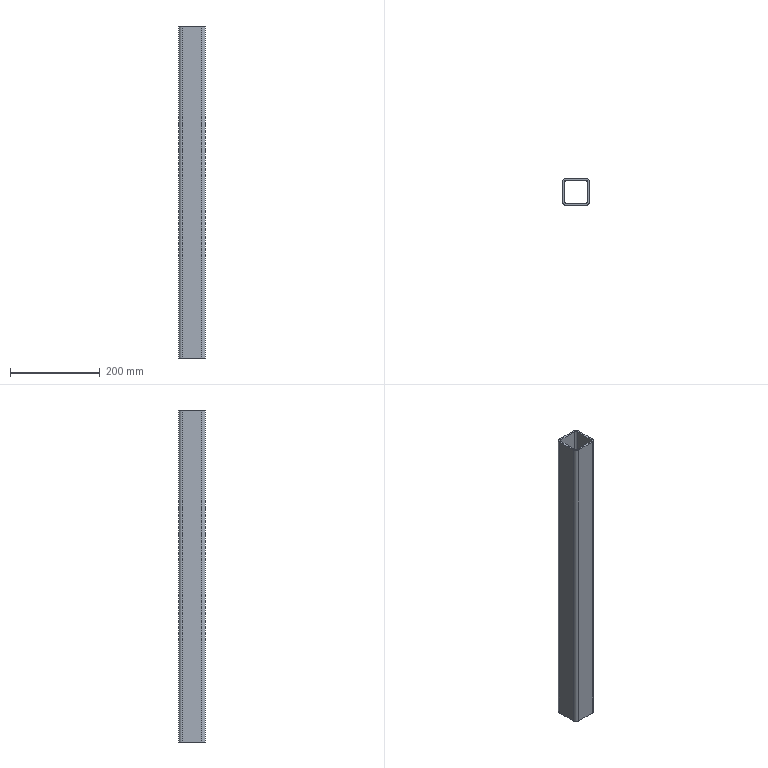Part | SolidWorks | features ICE 1, LibraryFeature 1 | 1 solid | 18 faces | box 60 x 60 x 740 mm | volume 632549 mm3 | plane 10 | cylinder 8 | commonest cylinder face diameters 8 x4 16 x4
STEP:
#1=CARTESIAN_POINT('',(22.,30.,0.));
#2=VERTEX_POINT('',#1);
#3=CARTESIAN_POINT('',(-22.,30.,0.));
#4=VERTEX_POINT('',#3);
#5=CARTESIAN_POINT('',(0.,30.,0.));
#6=DIRECTION('',(-1.,0.,0.));
#7=VECTOR('',#6,1000.);
#8=LINE('',#5,#7);
#9=EDGE_CURVE('',#2,#4,#8,.T.);
#10=ORIENTED_EDGE('',*,*,#9,.T.);
#11=CARTESIAN_POINT('',(-22.,30.,740.));
#12=VERTEX_POINT('',#11);
#13=CARTESIAN_POINT('',(-22.,30.,740.));
#14=DIRECTION('',(0.,0.,-1.));
#15=VECTOR('',#14,1000.);
#16=LINE('',#13,#15);
#17=EDGE_CURVE('',#12,#4,#16,.T.);
#18=ORIENTED_EDGE('',*,*,#17,.F.);
#19=CARTESIAN_POINT('',(22.,30.,740.));
#20=VERTEX_POINT('',#19);
#21=CARTESIAN_POINT('',(0.,30.,740.));
#22=DIRECTION('',(-1.,0.,0.));
#23=VECTOR('',#22,1000.);
#24=LINE('',#21,#23);
#25=EDGE_CURVE('',#20,#12,#24,.T.);
#26=ORIENTED_EDGE('',*,*,#25,.F.);
#27=CARTESIAN_POINT('',(22.,30.,740.));
#28=DIRECTION('',(0.,0.,-1.));
#29=VECTOR('',#28,1000.);
#30=LINE('',#27,#29);
#31=EDGE_CURVE('',#20,#2,#30,.T.);
#32=ORIENTED_EDGE('',*,*,#31,.T.);
#33=EDGE_LOOP('',(#10,#18,#26,#32));
#34=FACE_OUTER_BOUND('',#33,.T.);
#35=CARTESIAN_POINT('',(0.,30.,740.));
#36=DIRECTION('',(0.,-1.,0.));
#37=DIRECTION('',(0.,0.,-1.));
#38=AXIS2_PLACEMENT_3D('',#35,#36,#37);
#39=PLANE('',#38);
#40=ADVANCED_FACE('',(#34),#39,.F.);
#41=CARTESIAN_POINT('',(-30.,22.,0.));
#42=VERTEX_POINT('',#41);
#43=CARTESIAN_POINT('',(-22.,22.,0.));
#44=DIRECTION('',(0.,0.,1.));
#45=DIRECTION('',(1.,0.,0.));
#46=AXIS2_PLACEMENT_3D('',#43,#44,#45);
#47=CIRCLE('',#46,8.);
#48=EDGE_CURVE('',#4,#42,#47,.T.);
#49=ORIENTED_EDGE('',*,*,#48,.T.);
#50=CARTESIAN_POINT('',(-30.,22.,740.));
#51=VERTEX_POINT('',#50);
#52=CARTESIAN_POINT('',(-30.,22.,740.));
#53=DIRECTION('',(0.,0.,-1.));
#54=VECTOR('',#53,1000.);
#55=LINE('',#52,#54);
#56=EDGE_CURVE('',#51,#42,#55,.T.);
#57=ORIENTED_EDGE('',*,*,#56,.F.);
#58=CARTESIAN_POINT('',(-22.,22.,740.));
#59=DIRECTION('',(0.,0.,1.));
#60=DIRECTION('',(1.,0.,0.));
#61=AXIS2_PLACEMENT_3D('',#58,#59,#60);
#62=CIRCLE('',#61,8.);
#63=EDGE_CURVE('',#12,#51,#62,.T.);
#64=ORIENTED_EDGE('',*,*,#63,.F.);
#65=ORIENTED_EDGE('',*,*,#17,.T.);
#66=EDGE_LOOP('',(#49,#57,#64,#65));
#67=FACE_OUTER_BOUND('',#66,.T.);
#68=CARTESIAN_POINT('',(-22.,22.,740.));
#69=DIRECTION('',(0.,0.,-1.));
#70=DIRECTION('',(-1.,0.,0.));
#71=AXIS2_PLACEMENT_3D('',#68,#69,#70);
#72=CYLINDRICAL_SURFACE('',#71,8.);
#73=ADVANCED_FACE('',(#67),#72,.T.);
#74=CARTESIAN_POINT('',(-30.,-22.,0.));
#75=VERTEX_POINT('',#74);
#76=CARTESIAN_POINT('',(-30.,0.,0.));
#77=DIRECTION('',(0.,1.,0.));
#78=VECTOR('',#77,1000.);
#79=LINE('',#76,#78);
#80=EDGE_CURVE('',#75,#42,#79,.T.);
#81=ORIENTED_EDGE('',*,*,#80,.F.);
#82=CARTESIAN_POINT('',(-30.,-22.,740.));
#83=VERTEX_POINT('',#82);
#84=CARTESIAN_POINT('',(-30.,-22.,740.));
#85=DIRECTION('',(0.,0.,-1.));
#86=VECTOR('',#85,1000.);
#87=LINE('',#84,#86);
#88=EDGE_CURVE('',#83,#75,#87,.T.);
#89=ORIENTED_EDGE('',*,*,#88,.F.);
#90=CARTESIAN_POINT('',(-30.,0.,740.));
#91=DIRECTION('',(0.,1.,0.));
#92=VECTOR('',#91,1000.);
#93=LINE('',#90,#92);
#94=EDGE_CURVE('',#83,#51,#93,.T.);
#95=ORIENTED_EDGE('',*,*,#94,.T.);
#96=ORIENTED_EDGE('',*,*,#56,.T.);
#97=EDGE_LOOP('',(#81,#89,#95,#96));
#98=FACE_OUTER_BOUND('',#97,.T.);
#99=CARTESIAN_POINT('',(-30.,0.,740.));
#100=DIRECTION('',(-1.,0.,0.));
#101=DIRECTION('',(0.,0.,1.));
#102=AXIS2_PLACEMENT_3D('',#99,#100,#101);
#103=PLANE('',#102);
#104=ADVANCED_FACE('',(#98),#103,.T.);
#105=CARTESIAN_POINT('',(-22.,-30.,0.));
#106=VERTEX_POINT('',#105);
#107=CARTESIAN_POINT('',(-22.,-22.,0.));
#108=DIRECTION('',(0.,0.,1.));
#109=DIRECTION('',(1.,0.,0.));
#110=AXIS2_PLACEMENT_3D('',#107,#108,#109);
#111=CIRCLE('',#110,8.);
#112=EDGE_CURVE('',#75,#106,#111,.T.);
#113=ORIENTED_EDGE('',*,*,#112,.T.);
#114=CARTESIAN_POINT('',(-22.,-30.,740.));
#115=VERTEX_POINT('',#114);
#116=CARTESIAN_POINT('',(-22.,-30.,740.));
#117=DIRECTION('',(0.,0.,-1.));
#118=VECTOR('',#117,1000.);
#119=LINE('',#116,#118);
#120=EDGE_CURVE('',#115,#106,#119,.T.);
#121=ORIENTED_EDGE('',*,*,#120,.F.);
#122=CARTESIAN_POINT('',(-22.,-22.,740.));
#123=DIRECTION('',(0.,0.,1.));
#124=DIRECTION('',(1.,0.,0.));
#125=AXIS2_PLACEMENT_3D('',#122,#123,#124);
#126=CIRCLE('',#125,8.);
#127=EDGE_CURVE('',#83,#115,#126,.T.);
#128=ORIENTED_EDGE('',*,*,#127,.F.);
#129=ORIENTED_EDGE('',*,*,#88,.T.);
#130=EDGE_LOOP('',(#113,#121,#128,#129));
#131=FACE_OUTER_BOUND('',#130,.T.);
#132=CARTESIAN_POINT('',(-22.,-22.,740.));
#133=DIRECTION('',(0.,0.,-1.));
#134=DIRECTION('',(-1.,0.,0.));
#135=AXIS2_PLACEMENT_3D('',#132,#133,#134);
#136=CYLINDRICAL_SURFACE('',#135,8.);
#137=ADVANCED_FACE('',(#131),#136,.T.);
#138=CARTESIAN_POINT('',(22.,-30.,0.));
#139=VERTEX_POINT('',#138);
#140=CARTESIAN_POINT('',(0.,-30.,0.));
#141=DIRECTION('',(1.,0.,0.));
#142=VECTOR('',#141,1000.);
#143=LINE('',#140,#142);
#144=EDGE_CURVE('',#106,#139,#143,.T.);
#145=ORIENTED_EDGE('',*,*,#144,.T.);
#146=CARTESIAN_POINT('',(22.,-30.,740.));
#147=VERTEX_POINT('',#146);
#148=CARTESIAN_POINT('',(22.,-30.,740.));
#149=DIRECTION('',(0.,0.,-1.));
#150=VECTOR('',#149,1000.);
#151=LINE('',#148,#150);
#152=EDGE_CURVE('',#147,#139,#151,.T.);
#153=ORIENTED_EDGE('',*,*,#152,.F.);
#154=CARTESIAN_POINT('',(0.,-30.,740.));
#155=DIRECTION('',(1.,0.,0.));
#156=VECTOR('',#155,1000.);
#157=LINE('',#154,#156);
#158=EDGE_CURVE('',#115,#147,#157,.T.);
#159=ORIENTED_EDGE('',*,*,#158,.F.);
#160=ORIENTED_EDGE('',*,*,#120,.T.);
#161=EDGE_LOOP('',(#145,#153,#159,#160));
#162=FACE_OUTER_BOUND('',#161,.T.);
#163=CARTESIAN_POINT('',(0.,-30.,740.));
#164=DIRECTION('',(0.,1.,0.));
#165=DIRECTION('',(0.,0.,1.));
#166=AXIS2_PLACEMENT_3D('',#163,#164,#165);
#167=PLANE('',#166);
#168=ADVANCED_FACE('',(#162),#167,.F.);
#169=CARTESIAN_POINT('',(30.,-22.,0.));
#170=VERTEX_POINT('',#169);
#171=CARTESIAN_POINT('',(22.,-22.,0.));
#172=DIRECTION('',(0.,0.,1.));
#173=DIRECTION('',(1.,0.,0.));
#174=AXIS2_PLACEMENT_3D('',#171,#172,#173);
#175=CIRCLE('',#174,8.);
#176=EDGE_CURVE('',#139,#170,#175,.T.);
#177=ORIENTED_EDGE('',*,*,#176,.T.);
#178=CARTESIAN_POINT('',(30.,-22.,740.));
#179=VERTEX_POINT('',#178);
#180=CARTESIAN_POINT('',(30.,-22.,740.));
#181=DIRECTION('',(0.,0.,-1.));
#182=VECTOR('',#181,1000.);
#183=LINE('',#180,#182);
#184=EDGE_CURVE('',#179,#170,#183,.T.);
#185=ORIENTED_EDGE('',*,*,#184,.F.);
#186=CARTESIAN_POINT('',(22.,-22.,740.));
#187=DIRECTION('',(0.,0.,1.));
#188=DIRECTION('',(1.,0.,0.));
#189=AXIS2_PLACEMENT_3D('',#186,#187,#188);
#190=CIRCLE('',#189,8.);
#191=EDGE_CURVE('',#147,#179,#190,.T.);
#192=ORIENTED_EDGE('',*,*,#191,.F.);
#193=ORIENTED_EDGE('',*,*,#152,.T.);
#194=EDGE_LOOP('',(#177,#185,#192,#193));
#195=FACE_OUTER_BOUND('',#194,.T.);
#196=CARTESIAN_POINT('',(22.,-22.,740.));
#197=DIRECTION('',(0.,0.,-1.));
#198=DIRECTION('',(-1.,0.,0.));
#199=AXIS2_PLACEMENT_3D('',#196,#197,#198);
#200=CYLINDRICAL_SURFACE('',#199,8.);
#201=ADVANCED_FACE('',(#195),#200,.T.);
#202=CARTESIAN_POINT('',(30.,22.,0.));
#203=VERTEX_POINT('',#202);
#204=CARTESIAN_POINT('',(30.,0.,0.));
#205=DIRECTION('',(0.,-1.,0.));
#206=VECTOR('',#205,1000.);
#207=LINE('',#204,#206);
#208=EDGE_CURVE('',#203,#170,#207,.T.);
#209=ORIENTED_EDGE('',*,*,#208,.F.);
#210=CARTESIAN_POINT('',(30.,22.,740.));
#211=VERTEX_POINT('',#210);
#212=CARTESIAN_POINT('',(30.,22.,740.));
#213=DIRECTION('',(0.,0.,-1.));
#214=VECTOR('',#213,1000.);
#215=LINE('',#212,#214);
#216=EDGE_CURVE('',#211,#203,#215,.T.);
#217=ORIENTED_EDGE('',*,*,#216,.F.);
#218=CARTESIAN_POINT('',(30.,0.,740.));
#219=DIRECTION('',(0.,-1.,0.));
#220=VECTOR('',#219,1000.);
#221=LINE('',#218,#220);
#222=EDGE_CURVE('',#211,#179,#221,.T.);
#223=ORIENTED_EDGE('',*,*,#222,.T.);
#224=ORIENTED_EDGE('',*,*,#184,.T.);
#225=EDGE_LOOP('',(#209,#217,#223,#224));
#226=FACE_OUTER_BOUND('',#225,.T.);
#227=CARTESIAN_POINT('',(30.,0.,740.));
#228=DIRECTION('',(1.,0.,0.));
#229=DIRECTION('',(0.,0.,-1.));
#230=AXIS2_PLACEMENT_3D('',#227,#228,#229);
#231=PLANE('',#230);
#232=ADVANCED_FACE('',(#226),#231,.T.);
#233=CARTESIAN_POINT('',(-26.,-22.,0.));
#234=VERTEX_POINT('',#233);
#235=CARTESIAN_POINT('',(-22.,-26.,0.));
#236=VERTEX_POINT('',#235);
#237=CARTESIAN_POINT('',(-22.,-22.,0.));
#238=DIRECTION('',(0.,0.,1.));
#239=DIRECTION('',(1.,0.,0.));
#240=AXIS2_PLACEMENT_3D('',#237,#238,#239);
#241=CIRCLE('',#240,4.);
#242=EDGE_CURVE('',#234,#236,#241,.T.);
#243=ORIENTED_EDGE('',*,*,#242,.F.);
#244=CARTESIAN_POINT('',(-26.,-22.,740.));
#245=VERTEX_POINT('',#244);
#246=CARTESIAN_POINT('',(-26.,-22.,740.));
#247=DIRECTION('',(0.,0.,-1.));
#248=VECTOR('',#247,1000.);
#249=LINE('',#246,#248);
#250=EDGE_CURVE('',#245,#234,#249,.T.);
#251=ORIENTED_EDGE('',*,*,#250,.F.);
#252=CARTESIAN_POINT('',(-22.,-26.,740.));
#253=VERTEX_POINT('',#252);
#254=CARTESIAN_POINT('',(-22.,-22.,740.));
#255=DIRECTION('',(0.,0.,1.));
#256=DIRECTION('',(1.,0.,0.));
#257=AXIS2_PLACEMENT_3D('',#254,#255,#256);
#258=CIRCLE('',#257,4.);
#259=EDGE_CURVE('',#245,#253,#258,.T.);
#260=ORIENTED_EDGE('',*,*,#259,.T.);
#261=CARTESIAN_POINT('',(-22.,-26.,740.));
#262=DIRECTION('',(0.,0.,-1.));
#263=VECTOR('',#262,1000.);
#264=LINE('',#261,#263);
#265=EDGE_CURVE('',#253,#236,#264,.T.);
#266=ORIENTED_EDGE('',*,*,#265,.T.);
#267=EDGE_LOOP('',(#243,#251,#260,#266));
#268=FACE_OUTER_BOUND('',#267,.T.);
#269=CARTESIAN_POINT('',(-22.,-22.,740.));
#270=DIRECTION('',(0.,0.,-1.));
#271=DIRECTION('',(-1.,0.,0.));
#272=AXIS2_PLACEMENT_3D('',#269,#270,#271);
#273=CYLINDRICAL_SURFACE('',#272,4.);
#274=ADVANCED_FACE('',(#268),#273,.F.);
#275=CARTESIAN_POINT('',(-26.,22.,0.));
#276=VERTEX_POINT('',#275);
#277=CARTESIAN_POINT('',(-26.,0.,0.));
#278=DIRECTION('',(0.,1.,0.));
#279=VECTOR('',#278,1000.);
#280=LINE('',#277,#279);
#281=EDGE_CURVE('',#234,#276,#280,.T.);
#282=ORIENTED_EDGE('',*,*,#281,.T.);
#283=CARTESIAN_POINT('',(-26.,22.,740.));
#284=VERTEX_POINT('',#283);
#285=CARTESIAN_POINT('',(-26.,22.,740.));
#286=DIRECTION('',(0.,0.,-1.));
#287=VECTOR('',#286,1000.);
#288=LINE('',#285,#287);
#289=EDGE_CURVE('',#284,#276,#288,.T.);
#290=ORIENTED_EDGE('',*,*,#289,.F.);
#291=CARTESIAN_POINT('',(-26.,0.,740.));
#292=DIRECTION('',(0.,1.,0.));
#293=VECTOR('',#292,1000.);
#294=LINE('',#291,#293);
#295=EDGE_CURVE('',#245,#284,#294,.T.);
#296=ORIENTED_EDGE('',*,*,#295,.F.);
#297=ORIENTED_EDGE('',*,*,#250,.T.);
#298=EDGE_LOOP('',(#282,#290,#296,#297));
#299=FACE_OUTER_BOUND('',#298,.T.);
#300=CARTESIAN_POINT('',(-26.,0.,740.));
#301=DIRECTION('',(-1.,0.,0.));
#302=DIRECTION('',(0.,0.,1.));
#303=AXIS2_PLACEMENT_3D('',#300,#301,#302);
#304=PLANE('',#303);
#305=ADVANCED_FACE('',(#299),#304,.F.);
#306=CARTESIAN_POINT('',(-22.,26.,0.));
#307=VERTEX_POINT('',#306);
#308=CARTESIAN_POINT('',(-22.,22.,0.));
#309=DIRECTION('',(0.,0.,1.));
#310=DIRECTION('',(1.,0.,0.));
#311=AXIS2_PLACEMENT_3D('',#308,#309,#310);
#312=CIRCLE('',#311,4.);
#313=EDGE_CURVE('',#307,#276,#312,.T.);
#314=ORIENTED_EDGE('',*,*,#313,.F.);
#315=CARTESIAN_POINT('',(-22.,26.,740.));
#316=VERTEX_POINT('',#315);
#317=CARTESIAN_POINT('',(-22.,26.,740.));
#318=DIRECTION('',(0.,0.,-1.));
#319=VECTOR('',#318,1000.);
#320=LINE('',#317,#319);
#321=EDGE_CURVE('',#316,#307,#320,.T.);
#322=ORIENTED_EDGE('',*,*,#321,.F.);
#323=CARTESIAN_POINT('',(-22.,22.,740.));
#324=DIRECTION('',(0.,0.,1.));
#325=DIRECTION('',(1.,0.,0.));
#326=AXIS2_PLACEMENT_3D('',#323,#324,#325);
#327=CIRCLE('',#326,4.);
#328=EDGE_CURVE('',#316,#284,#327,.T.);
#329=ORIENTED_EDGE('',*,*,#328,.T.);
#330=ORIENTED_EDGE('',*,*,#289,.T.);
#331=EDGE_LOOP('',(#314,#322,#329,#330));
#332=FACE_OUTER_BOUND('',#331,.T.);
#333=CARTESIAN_POINT('',(-22.,22.,740.));
#334=DIRECTION('',(0.,0.,-1.));
#335=DIRECTION('',(-1.,0.,0.));
#336=AXIS2_PLACEMENT_3D('',#333,#334,#335);
#337=CYLINDRICAL_SURFACE('',#336,4.);
#338=ADVANCED_FACE('',(#332),#337,.F.);
#339=CARTESIAN_POINT('',(22.,26.,0.));
#340=VERTEX_POINT('',#339);
#341=CARTESIAN_POINT('',(0.,26.,0.));
#342=DIRECTION('',(-1.,0.,0.));
#343=VECTOR('',#342,1000.);
#344=LINE('',#341,#343);
#345=EDGE_CURVE('',#340,#307,#344,.T.);
#346=ORIENTED_EDGE('',*,*,#345,.F.);
#347=CARTESIAN_POINT('',(22.,26.,740.));
#348=VERTEX_POINT('',#347);
#349=CARTESIAN_POINT('',(22.,26.,740.));
#350=DIRECTION('',(0.,0.,-1.));
#351=VECTOR('',#350,1000.);
#352=LINE('',#349,#351);
#353=EDGE_CURVE('',#348,#340,#352,.T.);
#354=ORIENTED_EDGE('',*,*,#353,.F.);
#355=CARTESIAN_POINT('',(0.,26.,740.));
#356=DIRECTION('',(-1.,0.,0.));
#357=VECTOR('',#356,1000.);
#358=LINE('',#355,#357);
#359=EDGE_CURVE('',#348,#316,#358,.T.);
#360=ORIENTED_EDGE('',*,*,#359,.T.);
#361=ORIENTED_EDGE('',*,*,#321,.T.);
#362=EDGE_LOOP('',(#346,#354,#360,#361));
#363=FACE_OUTER_BOUND('',#362,.T.);
#364=CARTESIAN_POINT('',(0.,26.,740.));
#365=DIRECTION('',(0.,-1.,0.));
#366=DIRECTION('',(0.,0.,-1.));
#367=AXIS2_PLACEMENT_3D('',#364,#365,#366);
#368=PLANE('',#367);
#369=ADVANCED_FACE('',(#363),#368,.T.);
#370=CARTESIAN_POINT('',(26.,22.,0.));
#371=VERTEX_POINT('',#370);
#372=CARTESIAN_POINT('',(22.,22.,0.));
#373=DIRECTION('',(0.,0.,1.));
#374=DIRECTION('',(1.,0.,0.));
#375=AXIS2_PLACEMENT_3D('',#372,#373,#374);
#376=CIRCLE('',#375,4.);
#377=EDGE_CURVE('',#371,#340,#376,.T.);
#378=ORIENTED_EDGE('',*,*,#377,.F.);
#379=CARTESIAN_POINT('',(26.,22.,740.));
#380=VERTEX_POINT('',#379);
#381=CARTESIAN_POINT('',(26.,22.,740.));
#382=DIRECTION('',(0.,0.,-1.));
#383=VECTOR('',#382,1000.);
#384=LINE('',#381,#383);
#385=EDGE_CURVE('',#380,#371,#384,.T.);
#386=ORIENTED_EDGE('',*,*,#385,.F.);
#387=CARTESIAN_POINT('',(22.,22.,740.));
#388=DIRECTION('',(0.,0.,1.));
#389=DIRECTION('',(1.,0.,0.));
#390=AXIS2_PLACEMENT_3D('',#387,#388,#389);
#391=CIRCLE('',#390,4.);
#392=EDGE_CURVE('',#380,#348,#391,.T.);
#393=ORIENTED_EDGE('',*,*,#392,.T.);
#394=ORIENTED_EDGE('',*,*,#353,.T.);
#395=EDGE_LOOP('',(#378,#386,#393,#394));
#396=FACE_OUTER_BOUND('',#395,.T.);
#397=CARTESIAN_POINT('',(22.,22.,740.));
#398=DIRECTION('',(0.,0.,-1.));
#399=DIRECTION('',(-1.,0.,0.));
#400=AXIS2_PLACEMENT_3D('',#397,#398,#399);
#401=CYLINDRICAL_SURFACE('',#400,4.);
#402=ADVANCED_FACE('',(#396),#401,.F.);
#403=CARTESIAN_POINT('',(26.,-22.,0.));
#404=VERTEX_POINT('',#403);
#405=CARTESIAN_POINT('',(26.,0.,0.));
#406=DIRECTION('',(0.,-1.,0.));
#407=VECTOR('',#406,1000.);
#408=LINE('',#405,#407);
#409=EDGE_CURVE('',#371,#404,#408,.T.);
#410=ORIENTED_EDGE('',*,*,#409,.T.);
#411=CARTESIAN_POINT('',(26.,-22.,740.));
#412=VERTEX_POINT('',#411);
#413=CARTESIAN_POINT('',(26.,-22.,740.));
#414=DIRECTION('',(0.,0.,-1.));
#415=VECTOR('',#414,1000.);
#416=LINE('',#413,#415);
#417=EDGE_CURVE('',#412,#404,#416,.T.);
#418=ORIENTED_EDGE('',*,*,#417,.F.);
#419=CARTESIAN_POINT('',(26.,0.,740.));
#420=DIRECTION('',(0.,-1.,0.));
#421=VECTOR('',#420,1000.);
#422=LINE('',#419,#421);
#423=EDGE_CURVE('',#380,#412,#422,.T.);
#424=ORIENTED_EDGE('',*,*,#423,.F.);
#425=ORIENTED_EDGE('',*,*,#385,.T.);
#426=EDGE_LOOP('',(#410,#418,#424,#425));
#427=FACE_OUTER_BOUND('',#426,.T.);
#428=CARTESIAN_POINT('',(26.,0.,740.));
#429=DIRECTION('',(1.,0.,0.));
#430=DIRECTION('',(0.,0.,-1.));
#431=AXIS2_PLACEMENT_3D('',#428,#429,#430);
#432=PLANE('',#431);
#433=ADVANCED_FACE('',(#427),#432,.F.);
#434=CARTESIAN_POINT('',(22.,-26.,0.));
#435=VERTEX_POINT('',#434);
#436=CARTESIAN_POINT('',(22.,-22.,0.));
#437=DIRECTION('',(0.,0.,1.));
#438=DIRECTION('',(1.,0.,0.));
#439=AXIS2_PLACEMENT_3D('',#436,#437,#438);
#440=CIRCLE('',#439,4.);
#441=EDGE_CURVE('',#435,#404,#440,.T.);
#442=ORIENTED_EDGE('',*,*,#441,.F.);
#443=CARTESIAN_POINT('',(22.,-26.,740.));
#444=VERTEX_POINT('',#443);
#445=CARTESIAN_POINT('',(22.,-26.,740.));
#446=DIRECTION('',(0.,0.,-1.));
#447=VECTOR('',#446,1000.);
#448=LINE('',#445,#447);
#449=EDGE_CURVE('',#444,#435,#448,.T.);
#450=ORIENTED_EDGE('',*,*,#449,.F.);
#451=CARTESIAN_POINT('',(22.,-22.,740.));
#452=DIRECTION('',(0.,0.,1.));
#453=DIRECTION('',(1.,0.,0.));
#454=AXIS2_PLACEMENT_3D('',#451,#452,#453);
#455=CIRCLE('',#454,4.);
#456=EDGE_CURVE('',#444,#412,#455,.T.);
#457=ORIENTED_EDGE('',*,*,#456,.T.);
#458=ORIENTED_EDGE('',*,*,#417,.T.);
#459=EDGE_LOOP('',(#442,#450,#457,#458));
#460=FACE_OUTER_BOUND('',#459,.T.);
#461=CARTESIAN_POINT('',(22.,-22.,740.));
#462=DIRECTION('',(0.,0.,-1.));
#463=DIRECTION('',(-1.,0.,0.));
#464=AXIS2_PLACEMENT_3D('',#461,#462,#463);
#465=CYLINDRICAL_SURFACE('',#464,4.);
#466=ADVANCED_FACE('',(#460),#465,.F.);
#467=CARTESIAN_POINT('',(0.,-26.,0.));
#468=DIRECTION('',(1.,0.,0.));
#469=VECTOR('',#468,1000.);
#470=LINE('',#467,#469);
#471=EDGE_CURVE('',#236,#435,#470,.T.);
#472=ORIENTED_EDGE('',*,*,#471,.F.);
#473=ORIENTED_EDGE('',*,*,#265,.F.);
#474=CARTESIAN_POINT('',(0.,-26.,740.));
#475=DIRECTION('',(1.,0.,0.));
#476=VECTOR('',#475,1000.);
#477=LINE('',#474,#476);
#478=EDGE_CURVE('',#253,#444,#477,.T.);
#479=ORIENTED_EDGE('',*,*,#478,.T.);
#480=ORIENTED_EDGE('',*,*,#449,.T.);
#481=EDGE_LOOP('',(#472,#473,#479,#480));
#482=FACE_OUTER_BOUND('',#481,.T.);
#483=CARTESIAN_POINT('',(0.,-26.,740.));
#484=DIRECTION('',(0.,1.,0.));
#485=DIRECTION('',(0.,0.,1.));
#486=AXIS2_PLACEMENT_3D('',#483,#484,#485);
#487=PLANE('',#486);
#488=ADVANCED_FACE('',(#482),#487,.T.);
#489=CARTESIAN_POINT('',(22.,22.,0.));
#490=DIRECTION('',(0.,0.,1.));
#491=DIRECTION('',(1.,0.,0.));
#492=AXIS2_PLACEMENT_3D('',#489,#490,#491);
#493=CIRCLE('',#492,8.);
#494=EDGE_CURVE('',#203,#2,#493,.T.);
#495=ORIENTED_EDGE('',*,*,#494,.T.);
#496=ORIENTED_EDGE('',*,*,#31,.F.);
#497=CARTESIAN_POINT('',(22.,22.,740.));
#498=DIRECTION('',(0.,0.,1.));
#499=DIRECTION('',(1.,0.,0.));
#500=AXIS2_PLACEMENT_3D('',#497,#498,#499);
#501=CIRCLE('',#500,8.);
#502=EDGE_CURVE('',#211,#20,#501,.T.);
#503=ORIENTED_EDGE('',*,*,#502,.F.);
#504=ORIENTED_EDGE('',*,*,#216,.T.);
#505=EDGE_LOOP('',(#495,#496,#503,#504));
#506=FACE_OUTER_BOUND('',#505,.T.);
#507=CARTESIAN_POINT('',(22.,22.,740.));
#508=DIRECTION('',(0.,0.,-1.));
#509=DIRECTION('',(-1.,0.,0.));
#510=AXIS2_PLACEMENT_3D('',#507,#508,#509);
#511=CYLINDRICAL_SURFACE('',#510,8.);
#512=ADVANCED_FACE('',(#506),#511,.T.);
#513=ORIENTED_EDGE('',*,*,#259,.F.);
#514=ORIENTED_EDGE('',*,*,#295,.T.);
#515=ORIENTED_EDGE('',*,*,#328,.F.);
#516=ORIENTED_EDGE('',*,*,#359,.F.);
#517=ORIENTED_EDGE('',*,*,#392,.F.);
#518=ORIENTED_EDGE('',*,*,#423,.T.);
#519=ORIENTED_EDGE('',*,*,#456,.F.);
#520=ORIENTED_EDGE('',*,*,#478,.F.);
#521=EDGE_LOOP('',(#513,#514,#515,#516,#517,#518,#519,#520));
#522=FACE_BOUND('',#521,.T.);
#523=ORIENTED_EDGE('',*,*,#25,.T.);
#524=ORIENTED_EDGE('',*,*,#63,.T.);
#525=ORIENTED_EDGE('',*,*,#94,.F.);
#526=ORIENTED_EDGE('',*,*,#127,.T.);
#527=ORIENTED_EDGE('',*,*,#158,.T.);
#528=ORIENTED_EDGE('',*,*,#191,.T.);
#529=ORIENTED_EDGE('',*,*,#222,.F.);
#530=ORIENTED_EDGE('',*,*,#502,.T.);
#531=EDGE_LOOP('',(#523,#524,#525,#526,#527,#528,#529,#530));
#532=FACE_OUTER_BOUND('',#531,.T.);
#533=CARTESIAN_POINT('',(0.,0.,740.));
#534=DIRECTION('',(0.,0.,1.));
#535=DIRECTION('',(1.,0.,0.));
#536=AXIS2_PLACEMENT_3D('',#533,#534,#535);
#537=PLANE('',#536);
#538=ADVANCED_FACE('',(#522,#532),#537,.T.);
#539=ORIENTED_EDGE('',*,*,#242,.T.);
#540=ORIENTED_EDGE('',*,*,#471,.T.);
#541=ORIENTED_EDGE('',*,*,#441,.T.);
#542=ORIENTED_EDGE('',*,*,#409,.F.);
#543=ORIENTED_EDGE('',*,*,#377,.T.);
#544=ORIENTED_EDGE('',*,*,#345,.T.);
#545=ORIENTED_EDGE('',*,*,#313,.T.);
#546=ORIENTED_EDGE('',*,*,#281,.F.);
#547=EDGE_LOOP('',(#539,#540,#541,#542,#543,#544,#545,#546));
#548=FACE_BOUND('',#547,.T.);
#549=ORIENTED_EDGE('',*,*,#9,.F.);
#550=ORIENTED_EDGE('',*,*,#494,.F.);
#551=ORIENTED_EDGE('',*,*,#208,.T.);
#552=ORIENTED_EDGE('',*,*,#176,.F.);
#553=ORIENTED_EDGE('',*,*,#144,.F.);
#554=ORIENTED_EDGE('',*,*,#112,.F.);
#555=ORIENTED_EDGE('',*,*,#80,.T.);
#556=ORIENTED_EDGE('',*,*,#48,.F.);
#557=EDGE_LOOP('',(#549,#550,#551,#552,#553,#554,#555,#556));
#558=FACE_OUTER_BOUND('',#557,.T.);
#559=CARTESIAN_POINT('',(0.,0.,0.));
#560=DIRECTION('',(0.,0.,1.));
#561=DIRECTION('',(1.,0.,0.));
#562=AXIS2_PLACEMENT_3D('',#559,#560,#561);
#563=PLANE('',#562);
#564=ADVANCED_FACE('',(#548,#558),#563,.F.);
#565=CLOSED_SHELL('',(#40,#73,#104,#137,#168,#201,#232,#274,#305,#338,#369,#402,#433,#466,#488,#512,#538,#564));
#566=MANIFOLD_SOLID_BREP('',#565);
#567=CARTESIAN_POINT('',(0.,0.,0.));
#568=DIRECTION('',(0.,0.,1.));
#569=DIRECTION('',(1.,0.,0.));
#570=AXIS2_PLACEMENT_3D('',#567,#568,#569);
#571=(LENGTH_UNIT()NAMED_UNIT(*)SI_UNIT(.MILLI.,.METRE.));
#572=UNCERTAINTY_MEASURE_WITH_UNIT(LENGTH_MEASURE(0.00001),#571,'','');
#573=(NAMED_UNIT(*)PLANE_ANGLE_UNIT()SI_UNIT($,.RADIAN.));
#574=(NAMED_UNIT(*)SI_UNIT($,.STERADIAN.)SOLID_ANGLE_UNIT());
#575=(GEOMETRIC_REPRESENTATION_CONTEXT(3)GLOBAL_UNCERTAINTY_ASSIGNED_CONTEXT((#572))GLOBAL_UNIT_ASSIGNED_CONTEXT((#571,#573,#574))REPRESENTATION_CONTEXT('',''));
#576=ADVANCED_BREP_SHAPE_REPRESENTATION('',(#566,#570),#575);